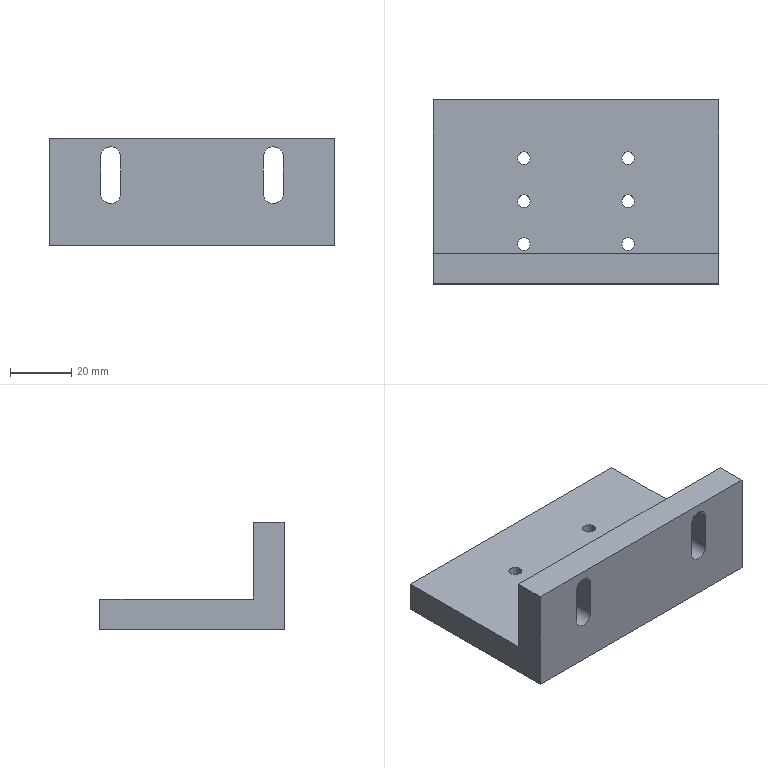CAM job | NX | 3+2 milling, drilling | part box 93 x 60 x 35 mm | stock box 98 x 65 x 40 mm
Tools:
number,name,description,diameter,corner_radius,flute_length,length,flutes
4,D4,平底铣刀-粗,4.0,0.0,25.0,75.0,2
9,D10,平底铣刀-粗,10.0,0.0,35.0,75.0,2
7,D6-J,平底铣刀-精,6.0,0.0,25.0,75.0,2
10,D10-J,平底铣刀-精,10.0,0.0,35.0,75.0,2
1,D80R0.8飞刀,圆鼻刀-粗,80.0,0.8,50.0,75.0,2
1,D80R0.8飞刀-J,圆鼻刀-精,80.0,0.8,50.0,75.0,2
2,D6倒角刀,倒角刀,6.0,0.0,3.0,25.0,2
22,M5X0.8,丝锥,4.2,0.0,35.0,50.0,2
14,ZT4.2,钻头,4.2,0.0,35.0,50.0,2
Operations:
program,operation,operation_type,tool,method,geometry_group,spindle_rpm,surface_speed,feed_per_tooth,feed_cut,feed_plunge,cut_length_mm,path_length_mm,cut_time_min,machine_time_min
C,底壁铣螺旋开粗-小_COPY,VolumeBased25DMillingOperation,D4,分层开粗-切深K-步距G,W-C,8000.0,100.528,0.125,2000.0,100.0,4467.066,4737.866,2.233,2.261
C,C0.3封闭铣廓倒角6X45L_COPY,PlanarMilling,D6倒角刀,爬面_倒角-切深0-步距G,W-C,7000.0,131.0,0.1071,1500.0,100.0,106.511,356.621,0.071,0.096
C,底壁铣螺旋精光-小_COPY,VolumeBased25DMillingOperation,D6-J,螺旋精光-切深K-步距G,W-C,8000.0,100.528,0.05,800.0,100.0,380.973,653.003,0.4762,0.5034
B,底壁铣飞面一刀开粗_COPY,VolumeBased25DMillingOperation,D80R0.8飞刀,分层开粗-切深K-步距G,W-B,2800.0,703.696,0.5357,3000.0,100.0,1810.746,3586.966,0.6036,0.7812
B,底壁铣飞面一刀精光_COPY,VolumeBased25DMillingOperation,D80R0.8飞刀-J,侧刃精光-切深K-步距G,W-B,4000.0,1005.28,0.125,1000.0,100.0,200.998,236.998,0.201,0.2046
B,底壁铣分层开粗-中_COPY,VolumeBased25DMillingOperation,D10,分层开粗-切深K-步距G,W-B,8000.0,251.327,0.3125,5000.0,100.0,32338.298,37228.514,6.468,6.957
B,钻倒角_1,Operation,D6倒角刀,METHOD,W-B,8000.0,150.796,0.0625,1000.0,0.0,22.668,207.104,0.0227,0.0411
B,C0.3平面去毛刺6X45L__COPY,SurfaceContour,D6倒角刀,爬面_倒角-切深0-步距G,W-B,8000.0,150.796,0.0938,1500.0,90.0,603.874,1191.896,0.4088,0.4676
B,底壁铣精光底面-中_COPY,VolumeBased25DMillingOperation,D10-J,精光步距切深关,W-B,7000.0,175.0,0.0536,1500.0,100.0,1179.685,1255.685,0.7865,0.7941
B,底壁铣精光侧面-中-选底面_COPY,VolumeBased25DMillingOperation,D10-J,侧刃精光-切深K-步距G,W-B,8000.0,251.32,0.0625,1000.0,100.0,223.363,395.591,0.2234,0.2406
A,顶面,FaceMilling,D80R0.8飞刀,侧刃精光-切深K-步距G,W-A,4000.0,1005.31,0.125,1000.0,100.0,187.0,223.0,0.187,0.1906
A,外形粗_2,VolumeBased25DMillingOperation,D10,METHOD,W-A,8000.0,251.327,0.3125,5000.0,80.0,15551.577,15625.077,3.11,3.118
A,打点-深0.8,Operation,D6倒角刀,NONE,W-A,8000.0,150.796,0.0312,500.0,90.0,10.8,156.757,0.0216,0.0362
A,通孔-M5螺纹底孔,Operation,ZT4.2,NONE,W-A,3000.0,38.924,0.0583,350.0,90.0,108.0,351.157,0.3086,0.3329
A,仅选体,SurfaceContour,D6倒角刀,METHOD,W-A,8000.0,150.796,0.1875,3000.0,100.0,323.315,359.116,0.1078,0.1114
A,铣倒角_1,PlanarMilling,D6倒角刀,METHOD,W-A,8000.0,150.796,0.0312,500.0,100.0,107.226,443.252,0.2145,0.2481
A,通孔-攻牙M5,Operation,M5X0.8,METHOD,W-A,500.0,6.597,0.0008,0.8,90.0,84.0,303.157,105.0,105.022
A,外形半精_2,VolumeBased25DMillingOperation,D10-J,METHOD,W-A,8000.0,251.327,0.0625,1000.0,100.0,684.748,870.263,0.6847,0.7033